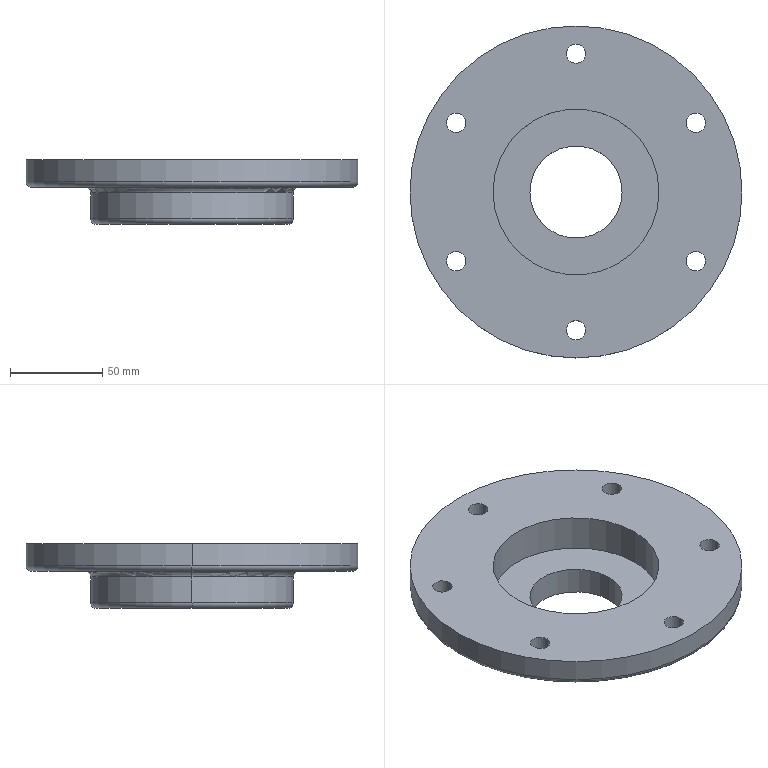Part | SolidWorks | features ICE 2, Extrusion 1, Fillet 1 | 1 solid | 30 faces | box 180 x 180 x 35 mm | volume 406222 mm3 | cylinder 20 | torus 6 | plane 4 | commonest cylinder face diameters 10.5 x12 50 x2 90 x2 110 x2 180 x2
STEP:
#1=CARTESIAN_POINT('',(55.,0.,-17.));
#2=VERTEX_POINT('',#1);
#3=CARTESIAN_POINT('',(-55.,0.,-17.));
#4=VERTEX_POINT('',#3);
#5=CARTESIAN_POINT('',(0.,0.,-17.));
#6=DIRECTION('',(0.,0.,1.));
#7=DIRECTION('',(-1.,0.,0.));
#8=AXIS2_PLACEMENT_3D('',#5,#6,#7);
#9=CIRCLE('',#8,55.);
#10=EDGE_CURVE('',#2,#4,#9,.T.);
#11=ORIENTED_EDGE('',*,*,#10,.F.);
#12=CARTESIAN_POINT('',(52.,0.,-20.));
#13=VERTEX_POINT('',#12);
#14=CARTESIAN_POINT('',(52.,0.,-17.));
#15=DIRECTION('',(0.,1.,0.));
#16=DIRECTION('',(-1.,0.,0.));
#17=AXIS2_PLACEMENT_3D('',#14,#15,#16);
#18=CIRCLE('',#17,3.);
#19=EDGE_CURVE('',#2,#13,#18,.T.);
#20=ORIENTED_EDGE('',*,*,#19,.T.);
#21=CARTESIAN_POINT('',(-52.,0.,-20.));
#22=VERTEX_POINT('',#21);
#23=CARTESIAN_POINT('',(0.,0.,-20.));
#24=DIRECTION('',(0.,0.,-1.));
#25=DIRECTION('',(-1.,0.,0.));
#26=AXIS2_PLACEMENT_3D('',#23,#24,#25);
#27=CIRCLE('',#26,52.);
#28=EDGE_CURVE('',#22,#13,#27,.T.);
#29=ORIENTED_EDGE('',*,*,#28,.F.);
#30=CARTESIAN_POINT('',(-52.,0.,-17.));
#31=DIRECTION('',(0.,-1.,0.));
#32=DIRECTION('',(0.,0.,-1.));
#33=AXIS2_PLACEMENT_3D('',#30,#31,#32);
#34=CIRCLE('',#33,3.);
#35=EDGE_CURVE('',#4,#22,#34,.T.);
#36=ORIENTED_EDGE('',*,*,#35,.F.);
#37=EDGE_LOOP('',(#11,#20,#29,#36));
#38=FACE_OUTER_BOUND('',#37,.T.);
#39=CARTESIAN_POINT('',(0.,0.,-17.));
#40=DIRECTION('',(0.,0.,-1.));
#41=DIRECTION('',(-1.,0.,0.));
#42=AXIS2_PLACEMENT_3D('',#39,#40,#41);
#43=TOROIDAL_SURFACE('',#42,52.,3.);
#44=ADVANCED_FACE('',(#38),#43,.T.);
#45=CARTESIAN_POINT('',(-87.,0.,0.));
#46=VERTEX_POINT('',#45);
#47=CARTESIAN_POINT('',(87.,0.,0.));
#48=VERTEX_POINT('',#47);
#49=CARTESIAN_POINT('',(0.,0.,0.));
#50=DIRECTION('',(0.,0.,-1.));
#51=DIRECTION('',(1.,0.,0.));
#52=AXIS2_PLACEMENT_3D('',#49,#50,#51);
#53=CIRCLE('',#52,87.);
#54=EDGE_CURVE('',#46,#48,#53,.T.);
#55=ORIENTED_EDGE('',*,*,#54,.F.);
#56=CARTESIAN_POINT('',(-90.,0.,3.));
#57=VERTEX_POINT('',#56);
#58=CARTESIAN_POINT('',(-87.,0.,3.));
#59=DIRECTION('',(0.,1.,0.));
#60=DIRECTION('',(-1.,0.,0.));
#61=AXIS2_PLACEMENT_3D('',#58,#59,#60);
#62=CIRCLE('',#61,3.);
#63=EDGE_CURVE('',#46,#57,#62,.T.);
#64=ORIENTED_EDGE('',*,*,#63,.T.);
#65=CARTESIAN_POINT('',(90.,0.,3.));
#66=VERTEX_POINT('',#65);
#67=CARTESIAN_POINT('',(0.,0.,3.));
#68=DIRECTION('',(0.,0.,1.));
#69=DIRECTION('',(1.,0.,0.));
#70=AXIS2_PLACEMENT_3D('',#67,#68,#69);
#71=CIRCLE('',#70,90.);
#72=EDGE_CURVE('',#66,#57,#71,.T.);
#73=ORIENTED_EDGE('',*,*,#72,.F.);
#74=CARTESIAN_POINT('',(87.,0.,3.));
#75=DIRECTION('',(0.,-1.,0.));
#76=DIRECTION('',(0.,0.,-1.));
#77=AXIS2_PLACEMENT_3D('',#74,#75,#76);
#78=CIRCLE('',#77,3.);
#79=EDGE_CURVE('',#48,#66,#78,.T.);
#80=ORIENTED_EDGE('',*,*,#79,.F.);
#81=EDGE_LOOP('',(#55,#64,#73,#80));
#82=FACE_OUTER_BOUND('',#81,.T.);
#83=CARTESIAN_POINT('',(0.,0.,3.));
#84=DIRECTION('',(0.,0.,1.));
#85=DIRECTION('',(1.,0.,0.));
#86=AXIS2_PLACEMENT_3D('',#83,#84,#85);
#87=TOROIDAL_SURFACE('',#86,87.,3.);
#88=ADVANCED_FACE('',(#82),#87,.T.);
#89=CARTESIAN_POINT('',(-58.,0.,0.));
#90=VERTEX_POINT('',#89);
#91=CARTESIAN_POINT('',(58.,0.,0.));
#92=VERTEX_POINT('',#91);
#93=CARTESIAN_POINT('',(0.,0.,0.));
#94=DIRECTION('',(0.,0.,1.));
#95=DIRECTION('',(1.,0.,0.));
#96=AXIS2_PLACEMENT_3D('',#93,#94,#95);
#97=CIRCLE('',#96,58.);
#98=EDGE_CURVE('',#90,#92,#97,.T.);
#99=ORIENTED_EDGE('',*,*,#98,.F.);
#100=CARTESIAN_POINT('',(-55.,0.,-3.));
#101=VERTEX_POINT('',#100);
#102=CARTESIAN_POINT('',(-58.,0.,-3.));
#103=DIRECTION('',(0.,1.,0.));
#104=DIRECTION('',(-1.,0.,0.));
#105=AXIS2_PLACEMENT_3D('',#102,#103,#104);
#106=CIRCLE('',#105,3.);
#107=EDGE_CURVE('',#90,#101,#106,.T.);
#108=ORIENTED_EDGE('',*,*,#107,.T.);
#109=CARTESIAN_POINT('',(55.,0.,-3.));
#110=VERTEX_POINT('',#109);
#111=CARTESIAN_POINT('',(0.,0.,-3.));
#112=DIRECTION('',(0.,0.,-1.));
#113=DIRECTION('',(1.,0.,0.));
#114=AXIS2_PLACEMENT_3D('',#111,#112,#113);
#115=CIRCLE('',#114,55.);
#116=EDGE_CURVE('',#110,#101,#115,.T.);
#117=ORIENTED_EDGE('',*,*,#116,.F.);
#118=CARTESIAN_POINT('',(58.,0.,-3.));
#119=DIRECTION('',(0.,-1.,0.));
#120=DIRECTION('',(0.,0.,-1.));
#121=AXIS2_PLACEMENT_3D('',#118,#119,#120);
#122=CIRCLE('',#121,3.);
#123=EDGE_CURVE('',#92,#110,#122,.T.);
#124=ORIENTED_EDGE('',*,*,#123,.F.);
#125=EDGE_LOOP('',(#99,#108,#117,#124));
#126=FACE_OUTER_BOUND('',#125,.T.);
#127=CARTESIAN_POINT('',(0.,0.,-3.));
#128=DIRECTION('',(0.,0.,1.));
#129=DIRECTION('',(1.,0.,0.));
#130=AXIS2_PLACEMENT_3D('',#127,#128,#129);
#131=TOROIDAL_SURFACE('',#130,58.,3.);
#132=ADVANCED_FACE('',(#126),#131,.F.);
#133=CARTESIAN_POINT('',(-45.,0.,-5.));
#134=VERTEX_POINT('',#133);
#135=CARTESIAN_POINT('',(45.,0.,-5.));
#136=VERTEX_POINT('',#135);
#137=CARTESIAN_POINT('',(0.,0.,-5.));
#138=DIRECTION('',(0.,0.,1.));
#139=DIRECTION('',(1.,0.,0.));
#140=AXIS2_PLACEMENT_3D('',#137,#138,#139);
#141=CIRCLE('',#140,45.);
#142=EDGE_CURVE('',#134,#136,#141,.T.);
#143=ORIENTED_EDGE('',*,*,#142,.F.);
#144=CARTESIAN_POINT('',(-45.,0.,15.));
#145=VERTEX_POINT('',#144);
#146=CARTESIAN_POINT('',(-45.,0.,-5.));
#147=DIRECTION('',(0.,0.,1.));
#148=VECTOR('',#147,1000.);
#149=LINE('',#146,#148);
#150=EDGE_CURVE('',#134,#145,#149,.T.);
#151=ORIENTED_EDGE('',*,*,#150,.T.);
#152=CARTESIAN_POINT('',(45.,0.,15.));
#153=VERTEX_POINT('',#152);
#154=CARTESIAN_POINT('',(0.,0.,15.));
#155=DIRECTION('',(0.,0.,1.));
#156=DIRECTION('',(1.,0.,0.));
#157=AXIS2_PLACEMENT_3D('',#154,#155,#156);
#158=CIRCLE('',#157,45.);
#159=EDGE_CURVE('',#145,#153,#158,.T.);
#160=ORIENTED_EDGE('',*,*,#159,.T.);
#161=CARTESIAN_POINT('',(45.,0.,-5.));
#162=DIRECTION('',(0.,0.,1.));
#163=VECTOR('',#162,1000.);
#164=LINE('',#161,#163);
#165=EDGE_CURVE('',#136,#153,#164,.T.);
#166=ORIENTED_EDGE('',*,*,#165,.F.);
#167=EDGE_LOOP('',(#143,#151,#160,#166));
#168=FACE_OUTER_BOUND('',#167,.T.);
#169=CARTESIAN_POINT('',(0.,0.,-5.));
#170=DIRECTION('',(0.,0.,1.));
#171=DIRECTION('',(1.,0.,0.));
#172=AXIS2_PLACEMENT_3D('',#169,#170,#171);
#173=CYLINDRICAL_SURFACE('',#172,45.);
#174=ADVANCED_FACE('',(#168),#173,.F.);
#175=ORIENTED_EDGE('',*,*,#10,.T.);
#176=CARTESIAN_POINT('',(-55.,0.,-20.));
#177=DIRECTION('',(0.,0.,1.));
#178=VECTOR('',#177,1000.);
#179=LINE('',#176,#178);
#180=EDGE_CURVE('',#4,#101,#179,.T.);
#181=ORIENTED_EDGE('',*,*,#180,.T.);
#182=CARTESIAN_POINT('',(0.,0.,-3.));
#183=DIRECTION('',(0.,0.,-1.));
#184=DIRECTION('',(1.,0.,0.));
#185=AXIS2_PLACEMENT_3D('',#182,#183,#184);
#186=CIRCLE('',#185,55.);
#187=EDGE_CURVE('',#101,#110,#186,.T.);
#188=ORIENTED_EDGE('',*,*,#187,.T.);
#189=CARTESIAN_POINT('',(55.,0.,-20.));
#190=DIRECTION('',(0.,0.,1.));
#191=VECTOR('',#190,1000.);
#192=LINE('',#189,#191);
#193=EDGE_CURVE('',#2,#110,#192,.T.);
#194=ORIENTED_EDGE('',*,*,#193,.F.);
#195=EDGE_LOOP('',(#175,#181,#188,#194));
#196=FACE_OUTER_BOUND('',#195,.T.);
#197=CARTESIAN_POINT('',(0.,0.,-20.));
#198=DIRECTION('',(0.,0.,1.));
#199=DIRECTION('',(1.,0.,0.));
#200=AXIS2_PLACEMENT_3D('',#197,#198,#199);
#201=CYLINDRICAL_SURFACE('',#200,55.);
#202=ADVANCED_FACE('',(#196),#201,.T.);
#203=CARTESIAN_POINT('',(-70.202,37.5,15.));
#204=VERTEX_POINT('',#203);
#205=CARTESIAN_POINT('',(-59.702,37.5,15.));
#206=VERTEX_POINT('',#205);
#207=CARTESIAN_POINT('',(-64.952,37.5,15.));
#208=DIRECTION('',(0.,0.,1.));
#209=DIRECTION('',(1.,0.,0.));
#210=AXIS2_PLACEMENT_3D('',#207,#208,#209);
#211=CIRCLE('',#210,5.25);
#212=EDGE_CURVE('',#204,#206,#211,.T.);
#213=ORIENTED_EDGE('',*,*,#212,.T.);
#214=CARTESIAN_POINT('',(-59.702,37.5,0.));
#215=VERTEX_POINT('',#214);
#216=CARTESIAN_POINT('',(-59.702,37.5,15.));
#217=DIRECTION('',(0.,0.,-1.));
#218=VECTOR('',#217,1000.);
#219=LINE('',#216,#218);
#220=EDGE_CURVE('',#206,#215,#219,.T.);
#221=ORIENTED_EDGE('',*,*,#220,.T.);
#222=CARTESIAN_POINT('',(-70.202,37.5,0.));
#223=VERTEX_POINT('',#222);
#224=CARTESIAN_POINT('',(-64.952,37.5,0.));
#225=DIRECTION('',(0.,0.,1.));
#226=DIRECTION('',(1.,0.,0.));
#227=AXIS2_PLACEMENT_3D('',#224,#225,#226);
#228=CIRCLE('',#227,5.25);
#229=EDGE_CURVE('',#223,#215,#228,.T.);
#230=ORIENTED_EDGE('',*,*,#229,.F.);
#231=CARTESIAN_POINT('',(-70.202,37.5,15.));
#232=DIRECTION('',(0.,0.,-1.));
#233=VECTOR('',#232,1000.);
#234=LINE('',#231,#233);
#235=EDGE_CURVE('',#204,#223,#234,.T.);
#236=ORIENTED_EDGE('',*,*,#235,.F.);
#237=EDGE_LOOP('',(#213,#221,#230,#236));
#238=FACE_OUTER_BOUND('',#237,.T.);
#239=CARTESIAN_POINT('',(-64.952,37.5,15.));
#240=DIRECTION('',(0.,0.,-1.));
#241=DIRECTION('',(-1.,0.,0.));
#242=AXIS2_PLACEMENT_3D('',#239,#240,#241);
#243=CYLINDRICAL_SURFACE('',#242,5.25);
#244=ADVANCED_FACE('',(#238),#243,.F.);
#245=CARTESIAN_POINT('',(-70.202,-37.5,15.));
#246=VERTEX_POINT('',#245);
#247=CARTESIAN_POINT('',(-59.702,-37.5,15.));
#248=VERTEX_POINT('',#247);
#249=CARTESIAN_POINT('',(-64.952,-37.5,15.));
#250=DIRECTION('',(0.,0.,1.));
#251=DIRECTION('',(1.,0.,0.));
#252=AXIS2_PLACEMENT_3D('',#249,#250,#251);
#253=CIRCLE('',#252,5.25);
#254=EDGE_CURVE('',#246,#248,#253,.T.);
#255=ORIENTED_EDGE('',*,*,#254,.T.);
#256=CARTESIAN_POINT('',(-59.702,-37.5,0.));
#257=VERTEX_POINT('',#256);
#258=CARTESIAN_POINT('',(-59.702,-37.5,15.));
#259=DIRECTION('',(0.,0.,-1.));
#260=VECTOR('',#259,1000.);
#261=LINE('',#258,#260);
#262=EDGE_CURVE('',#248,#257,#261,.T.);
#263=ORIENTED_EDGE('',*,*,#262,.T.);
#264=CARTESIAN_POINT('',(-70.202,-37.5,0.));
#265=VERTEX_POINT('',#264);
#266=CARTESIAN_POINT('',(-64.952,-37.5,0.));
#267=DIRECTION('',(0.,0.,1.));
#268=DIRECTION('',(1.,0.,0.));
#269=AXIS2_PLACEMENT_3D('',#266,#267,#268);
#270=CIRCLE('',#269,5.25);
#271=EDGE_CURVE('',#265,#257,#270,.T.);
#272=ORIENTED_EDGE('',*,*,#271,.F.);
#273=CARTESIAN_POINT('',(-70.202,-37.5,15.));
#274=DIRECTION('',(0.,0.,-1.));
#275=VECTOR('',#274,1000.);
#276=LINE('',#273,#275);
#277=EDGE_CURVE('',#246,#265,#276,.T.);
#278=ORIENTED_EDGE('',*,*,#277,.F.);
#279=EDGE_LOOP('',(#255,#263,#272,#278));
#280=FACE_OUTER_BOUND('',#279,.T.);
#281=CARTESIAN_POINT('',(-64.952,-37.5,15.));
#282=DIRECTION('',(0.,0.,-1.));
#283=DIRECTION('',(-1.,0.,0.));
#284=AXIS2_PLACEMENT_3D('',#281,#282,#283);
#285=CYLINDRICAL_SURFACE('',#284,5.25);
#286=ADVANCED_FACE('',(#280),#285,.F.);
#287=CARTESIAN_POINT('',(-5.25,-75.,15.));
#288=VERTEX_POINT('',#287);
#289=CARTESIAN_POINT('',(5.25,-75.,15.));
#290=VERTEX_POINT('',#289);
#291=CARTESIAN_POINT('',(0.,-75.,15.));
#292=DIRECTION('',(0.,0.,1.));
#293=DIRECTION('',(1.,0.,0.));
#294=AXIS2_PLACEMENT_3D('',#291,#292,#293);
#295=CIRCLE('',#294,5.25);
#296=EDGE_CURVE('',#288,#290,#295,.T.);
#297=ORIENTED_EDGE('',*,*,#296,.T.);
#298=CARTESIAN_POINT('',(5.25,-75.,0.));
#299=VERTEX_POINT('',#298);
#300=CARTESIAN_POINT('',(5.25,-75.,15.));
#301=DIRECTION('',(0.,0.,-1.));
#302=VECTOR('',#301,1000.);
#303=LINE('',#300,#302);
#304=EDGE_CURVE('',#290,#299,#303,.T.);
#305=ORIENTED_EDGE('',*,*,#304,.T.);
#306=CARTESIAN_POINT('',(-5.25,-75.,0.));
#307=VERTEX_POINT('',#306);
#308=CARTESIAN_POINT('',(0.,-75.,0.));
#309=DIRECTION('',(0.,0.,1.));
#310=DIRECTION('',(1.,0.,0.));
#311=AXIS2_PLACEMENT_3D('',#308,#309,#310);
#312=CIRCLE('',#311,5.25);
#313=EDGE_CURVE('',#307,#299,#312,.T.);
#314=ORIENTED_EDGE('',*,*,#313,.F.);
#315=CARTESIAN_POINT('',(-5.25,-75.,15.));
#316=DIRECTION('',(0.,0.,-1.));
#317=VECTOR('',#316,1000.);
#318=LINE('',#315,#317);
#319=EDGE_CURVE('',#288,#307,#318,.T.);
#320=ORIENTED_EDGE('',*,*,#319,.F.);
#321=EDGE_LOOP('',(#297,#305,#314,#320));
#322=FACE_OUTER_BOUND('',#321,.T.);
#323=CARTESIAN_POINT('',(0.,-75.,15.));
#324=DIRECTION('',(0.,0.,-1.));
#325=DIRECTION('',(-1.,0.,0.));
#326=AXIS2_PLACEMENT_3D('',#323,#324,#325);
#327=CYLINDRICAL_SURFACE('',#326,5.25);
#328=ADVANCED_FACE('',(#322),#327,.F.);
#329=CARTESIAN_POINT('',(59.702,-37.5,15.));
#330=VERTEX_POINT('',#329);
#331=CARTESIAN_POINT('',(70.202,-37.5,15.));
#332=VERTEX_POINT('',#331);
#333=CARTESIAN_POINT('',(64.952,-37.5,15.));
#334=DIRECTION('',(0.,0.,1.));
#335=DIRECTION('',(1.,0.,0.));
#336=AXIS2_PLACEMENT_3D('',#333,#334,#335);
#337=CIRCLE('',#336,5.25);
#338=EDGE_CURVE('',#330,#332,#337,.T.);
#339=ORIENTED_EDGE('',*,*,#338,.T.);
#340=CARTESIAN_POINT('',(70.202,-37.5,0.));
#341=VERTEX_POINT('',#340);
#342=CARTESIAN_POINT('',(70.202,-37.5,15.));
#343=DIRECTION('',(0.,0.,-1.));
#344=VECTOR('',#343,1000.);
#345=LINE('',#342,#344);
#346=EDGE_CURVE('',#332,#341,#345,.T.);
#347=ORIENTED_EDGE('',*,*,#346,.T.);
#348=CARTESIAN_POINT('',(59.702,-37.5,0.));
#349=VERTEX_POINT('',#348);
#350=CARTESIAN_POINT('',(64.952,-37.5,0.));
#351=DIRECTION('',(0.,0.,1.));
#352=DIRECTION('',(1.,0.,0.));
#353=AXIS2_PLACEMENT_3D('',#350,#351,#352);
#354=CIRCLE('',#353,5.25);
#355=EDGE_CURVE('',#349,#341,#354,.T.);
#356=ORIENTED_EDGE('',*,*,#355,.F.);
#357=CARTESIAN_POINT('',(59.702,-37.5,15.));
#358=DIRECTION('',(0.,0.,-1.));
#359=VECTOR('',#358,1000.);
#360=LINE('',#357,#359);
#361=EDGE_CURVE('',#330,#349,#360,.T.);
#362=ORIENTED_EDGE('',*,*,#361,.F.);
#363=EDGE_LOOP('',(#339,#347,#356,#362));
#364=FACE_OUTER_BOUND('',#363,.T.);
#365=CARTESIAN_POINT('',(64.952,-37.5,15.));
#366=DIRECTION('',(0.,0.,-1.));
#367=DIRECTION('',(-1.,0.,0.));
#368=AXIS2_PLACEMENT_3D('',#365,#366,#367);
#369=CYLINDRICAL_SURFACE('',#368,5.25);
#370=ADVANCED_FACE('',(#364),#369,.F.);
#371=CARTESIAN_POINT('',(59.702,37.5,15.));
#372=VERTEX_POINT('',#371);
#373=CARTESIAN_POINT('',(70.202,37.5,15.));
#374=VERTEX_POINT('',#373);
#375=CARTESIAN_POINT('',(64.952,37.5,15.));
#376=DIRECTION('',(0.,0.,1.));
#377=DIRECTION('',(1.,0.,0.));
#378=AXIS2_PLACEMENT_3D('',#375,#376,#377);
#379=CIRCLE('',#378,5.25);
#380=EDGE_CURVE('',#372,#374,#379,.T.);
#381=ORIENTED_EDGE('',*,*,#380,.T.);
#382=CARTESIAN_POINT('',(70.202,37.5,0.));
#383=VERTEX_POINT('',#382);
#384=CARTESIAN_POINT('',(70.202,37.5,15.));
#385=DIRECTION('',(0.,0.,-1.));
#386=VECTOR('',#385,1000.);
#387=LINE('',#384,#386);
#388=EDGE_CURVE('',#374,#383,#387,.T.);
#389=ORIENTED_EDGE('',*,*,#388,.T.);
#390=CARTESIAN_POINT('',(59.702,37.5,0.));
#391=VERTEX_POINT('',#390);
#392=CARTESIAN_POINT('',(64.952,37.5,0.));
#393=DIRECTION('',(0.,0.,1.));
#394=DIRECTION('',(1.,0.,0.));
#395=AXIS2_PLACEMENT_3D('',#392,#393,#394);
#396=CIRCLE('',#395,5.25);
#397=EDGE_CURVE('',#391,#383,#396,.T.);
#398=ORIENTED_EDGE('',*,*,#397,.F.);
#399=CARTESIAN_POINT('',(59.702,37.5,15.));
#400=DIRECTION('',(0.,0.,-1.));
#401=VECTOR('',#400,1000.);
#402=LINE('',#399,#401);
#403=EDGE_CURVE('',#372,#391,#402,.T.);
#404=ORIENTED_EDGE('',*,*,#403,.F.);
#405=EDGE_LOOP('',(#381,#389,#398,#404));
#406=FACE_OUTER_BOUND('',#405,.T.);
#407=CARTESIAN_POINT('',(64.952,37.5,15.));
#408=DIRECTION('',(0.,0.,-1.));
#409=DIRECTION('',(-1.,0.,0.));
#410=AXIS2_PLACEMENT_3D('',#407,#408,#409);
#411=CYLINDRICAL_SURFACE('',#410,5.25);
#412=ADVANCED_FACE('',(#406),#411,.F.);
#413=CARTESIAN_POINT('',(-5.25,75.,15.));
#414=VERTEX_POINT('',#413);
#415=CARTESIAN_POINT('',(5.25,75.,15.));
#416=VERTEX_POINT('',#415);
#417=CARTESIAN_POINT('',(0.,75.,15.));
#418=DIRECTION('',(0.,0.,1.));
#419=DIRECTION('',(1.,0.,0.));
#420=AXIS2_PLACEMENT_3D('',#417,#418,#419);
#421=CIRCLE('',#420,5.25);
#422=EDGE_CURVE('',#414,#416,#421,.T.);
#423=ORIENTED_EDGE('',*,*,#422,.T.);
#424=CARTESIAN_POINT('',(5.25,75.,0.));
#425=VERTEX_POINT('',#424);
#426=CARTESIAN_POINT('',(5.25,75.,15.));
#427=DIRECTION('',(0.,0.,-1.));
#428=VECTOR('',#427,1000.);
#429=LINE('',#426,#428);
#430=EDGE_CURVE('',#416,#425,#429,.T.);
#431=ORIENTED_EDGE('',*,*,#430,.T.);
#432=CARTESIAN_POINT('',(-5.25,75.,0.));
#433=VERTEX_POINT('',#432);
#434=CARTESIAN_POINT('',(0.,75.,0.));
#435=DIRECTION('',(0.,0.,1.));
#436=DIRECTION('',(1.,0.,0.));
#437=AXIS2_PLACEMENT_3D('',#434,#435,#436);
#438=CIRCLE('',#437,5.25);
#439=EDGE_CURVE('',#433,#425,#438,.T.);
#440=ORIENTED_EDGE('',*,*,#439,.F.);
#441=CARTESIAN_POINT('',(-5.25,75.,15.));
#442=DIRECTION('',(0.,0.,-1.));
#443=VECTOR('',#442,1000.);
#444=LINE('',#441,#443);
#445=EDGE_CURVE('',#414,#433,#444,.T.);
#446=ORIENTED_EDGE('',*,*,#445,.F.);
#447=EDGE_LOOP('',(#423,#431,#440,#446));
#448=FACE_OUTER_BOUND('',#447,.T.);
#449=CARTESIAN_POINT('',(0.,75.,15.));
#450=DIRECTION('',(0.,0.,-1.));
#451=DIRECTION('',(-1.,0.,0.));
#452=AXIS2_PLACEMENT_3D('',#449,#450,#451);
#453=CYLINDRICAL_SURFACE('',#452,5.25);
#454=ADVANCED_FACE('',(#448),#453,.F.);
#455=CARTESIAN_POINT('',(90.,0.,15.));
#456=VERTEX_POINT('',#455);
#457=CARTESIAN_POINT('',(-90.,0.,15.));
#458=VERTEX_POINT('',#457);
#459=CARTESIAN_POINT('',(0.,0.,15.));
#460=DIRECTION('',(0.,0.,1.));
#461=DIRECTION('',(1.,0.,0.));
#462=AXIS2_PLACEMENT_3D('',#459,#460,#461);
#463=CIRCLE('',#462,90.);
#464=EDGE_CURVE('',#456,#458,#463,.T.);
#465=ORIENTED_EDGE('',*,*,#464,.F.);
#466=CARTESIAN_POINT('',(90.,0.,15.));
#467=DIRECTION('',(0.,0.,-1.));
#468=VECTOR('',#467,1000.);
#469=LINE('',#466,#468);
#470=EDGE_CURVE('',#456,#66,#469,.T.);
#471=ORIENTED_EDGE('',*,*,#470,.T.);
#472=ORIENTED_EDGE('',*,*,#72,.T.);
#473=CARTESIAN_POINT('',(-90.,0.,15.));
#474=DIRECTION('',(0.,0.,-1.));
#475=VECTOR('',#474,1000.);
#476=LINE('',#473,#475);
#477=EDGE_CURVE('',#458,#57,#476,.T.);
#478=ORIENTED_EDGE('',*,*,#477,.F.);
#479=EDGE_LOOP('',(#465,#471,#472,#478));
#480=FACE_OUTER_BOUND('',#479,.T.);
#481=CARTESIAN_POINT('',(0.,0.,15.));
#482=DIRECTION('',(0.,0.,-1.));
#483=DIRECTION('',(-1.,0.,0.));
#484=AXIS2_PLACEMENT_3D('',#481,#482,#483);
#485=CYLINDRICAL_SURFACE('',#484,90.);
#486=ADVANCED_FACE('',(#480),#485,.T.);
#487=CARTESIAN_POINT('',(-25.,0.,-5.));
#488=VERTEX_POINT('',#487);
#489=CARTESIAN_POINT('',(25.,0.,-5.));
#490=VERTEX_POINT('',#489);
#491=CARTESIAN_POINT('',(0.,0.,-5.));
#492=DIRECTION('',(0.,0.,1.));
#493=DIRECTION('',(1.,0.,0.));
#494=AXIS2_PLACEMENT_3D('',#491,#492,#493);
#495=CIRCLE('',#494,25.);
#496=EDGE_CURVE('',#488,#490,#495,.T.);
#497=ORIENTED_EDGE('',*,*,#496,.T.);
#498=CARTESIAN_POINT('',(25.,0.,-20.));
#499=VERTEX_POINT('',#498);
#500=CARTESIAN_POINT('',(25.,0.,15.));
#501=DIRECTION('',(0.,0.,-1.));
#502=VECTOR('',#501,1000.);
#503=LINE('',#500,#502);
#504=EDGE_CURVE('',#490,#499,#503,.T.);
#505=ORIENTED_EDGE('',*,*,#504,.T.);
#506=CARTESIAN_POINT('',(-25.,0.,-20.));
#507=VERTEX_POINT('',#506);
#508=CARTESIAN_POINT('',(0.,0.,-20.));
#509=DIRECTION('',(0.,0.,-1.));
#510=DIRECTION('',(-1.,0.,0.));
#511=AXIS2_PLACEMENT_3D('',#508,#509,#510);
#512=CIRCLE('',#511,25.);
#513=EDGE_CURVE('',#499,#507,#512,.T.);
#514=ORIENTED_EDGE('',*,*,#513,.T.);
#515=CARTESIAN_POINT('',(-25.,0.,15.));
#516=DIRECTION('',(0.,0.,-1.));
#517=VECTOR('',#516,1000.);
#518=LINE('',#515,#517);
#519=EDGE_CURVE('',#488,#507,#518,.T.);
#520=ORIENTED_EDGE('',*,*,#519,.F.);
#521=EDGE_LOOP('',(#497,#505,#514,#520));
#522=FACE_OUTER_BOUND('',#521,.T.);
#523=CARTESIAN_POINT('',(0.,0.,15.));
#524=DIRECTION('',(0.,0.,-1.));
#525=DIRECTION('',(-1.,0.,0.));
#526=AXIS2_PLACEMENT_3D('',#523,#524,#525);
#527=CYLINDRICAL_SURFACE('',#526,25.);
#528=ADVANCED_FACE('',(#522),#527,.F.);
#529=ORIENTED_EDGE('',*,*,#504,.F.);
#530=CARTESIAN_POINT('',(0.,0.,-5.));
#531=DIRECTION('',(0.,0.,1.));
#532=DIRECTION('',(1.,0.,0.));
#533=AXIS2_PLACEMENT_3D('',#530,#531,#532);
#534=CIRCLE('',#533,25.);
#535=EDGE_CURVE('',#490,#488,#534,.T.);
#536=ORIENTED_EDGE('',*,*,#535,.T.);
#537=ORIENTED_EDGE('',*,*,#519,.T.);
#538=CARTESIAN_POINT('',(0.,0.,-20.));
#539=DIRECTION('',(0.,0.,-1.));
#540=DIRECTION('',(-1.,0.,0.));
#541=AXIS2_PLACEMENT_3D('',#538,#539,#540);
#542=CIRCLE('',#541,25.);
#543=EDGE_CURVE('',#507,#499,#542,.T.);
#544=ORIENTED_EDGE('',*,*,#543,.T.);
#545=EDGE_LOOP('',(#529,#536,#537,#544));
#546=FACE_OUTER_BOUND('',#545,.T.);
#547=CARTESIAN_POINT('',(0.,0.,15.));
#548=DIRECTION('',(0.,0.,-1.));
#549=DIRECTION('',(-1.,0.,0.));
#550=AXIS2_PLACEMENT_3D('',#547,#548,#549);
#551=CYLINDRICAL_SURFACE('',#550,25.);
#552=ADVANCED_FACE('',(#546),#551,.F.);
#553=CARTESIAN_POINT('',(0.,0.,0.));
#554=DIRECTION('',(0.,0.,1.));
#555=DIRECTION('',(1.,0.,0.));
#556=AXIS2_PLACEMENT_3D('',#553,#554,#555);
#557=CIRCLE('',#556,58.);
#558=EDGE_CURVE('',#92,#90,#557,.T.);
#559=ORIENTED_EDGE('',*,*,#558,.T.);
#560=ORIENTED_EDGE('',*,*,#98,.T.);
#561=EDGE_LOOP('',(#559,#560));
#562=FACE_BOUND('',#561,.T.);
#563=CARTESIAN_POINT('',(0.,0.,0.));
#564=DIRECTION('',(0.,0.,-1.));
#565=DIRECTION('',(1.,0.,0.));
#566=AXIS2_PLACEMENT_3D('',#563,#564,#565);
#567=CIRCLE('',#566,87.);
#568=EDGE_CURVE('',#48,#46,#567,.T.);
#569=ORIENTED_EDGE('',*,*,#568,.T.);
#570=ORIENTED_EDGE('',*,*,#54,.T.);
#571=EDGE_LOOP('',(#569,#570));
#572=FACE_OUTER_BOUND('',#571,.T.);
#573=ORIENTED_EDGE('',*,*,#229,.T.);
#574=CARTESIAN_POINT('',(-64.952,37.5,0.));
#575=DIRECTION('',(0.,0.,1.));
#576=DIRECTION('',(1.,0.,0.));
#577=AXIS2_PLACEMENT_3D('',#574,#575,#576);
#578=CIRCLE('',#577,5.25);
#579=EDGE_CURVE('',#215,#223,#578,.T.);
#580=ORIENTED_EDGE('',*,*,#579,.T.);
#581=EDGE_LOOP('',(#573,#580));
#582=FACE_BOUND('',#581,.T.);
#583=ORIENTED_EDGE('',*,*,#271,.T.);
#584=CARTESIAN_POINT('',(-64.952,-37.5,0.));
#585=DIRECTION('',(0.,0.,1.));
#586=DIRECTION('',(1.,0.,0.));
#587=AXIS2_PLACEMENT_3D('',#584,#585,#586);
#588=CIRCLE('',#587,5.25);
#589=EDGE_CURVE('',#257,#265,#588,.T.);
#590=ORIENTED_EDGE('',*,*,#589,.T.);
#591=EDGE_LOOP('',(#583,#590));
#592=FACE_BOUND('',#591,.T.);
#593=ORIENTED_EDGE('',*,*,#313,.T.);
#594=CARTESIAN_POINT('',(0.,-75.,0.));
#595=DIRECTION('',(0.,0.,1.));
#596=DIRECTION('',(1.,0.,0.));
#597=AXIS2_PLACEMENT_3D('',#594,#595,#596);
#598=CIRCLE('',#597,5.25);
#599=EDGE_CURVE('',#299,#307,#598,.T.);
#600=ORIENTED_EDGE('',*,*,#599,.T.);
#601=EDGE_LOOP('',(#593,#600));
#602=FACE_BOUND('',#601,.T.);
#603=ORIENTED_EDGE('',*,*,#355,.T.);
#604=CARTESIAN_POINT('',(64.952,-37.5,0.));
#605=DIRECTION('',(0.,0.,1.));
#606=DIRECTION('',(1.,0.,0.));
#607=AXIS2_PLACEMENT_3D('',#604,#605,#606);
#608=CIRCLE('',#607,5.25);
#609=EDGE_CURVE('',#341,#349,#608,.T.);
#610=ORIENTED_EDGE('',*,*,#609,.T.);
#611=EDGE_LOOP('',(#603,#610));
#612=FACE_BOUND('',#611,.T.);
#613=ORIENTED_EDGE('',*,*,#397,.T.);
#614=CARTESIAN_POINT('',(64.952,37.5,0.));
#615=DIRECTION('',(0.,0.,1.));
#616=DIRECTION('',(1.,0.,0.));
#617=AXIS2_PLACEMENT_3D('',#614,#615,#616);
#618=CIRCLE('',#617,5.25);
#619=EDGE_CURVE('',#383,#391,#618,.T.);
#620=ORIENTED_EDGE('',*,*,#619,.T.);
#621=EDGE_LOOP('',(#613,#620));
#622=FACE_BOUND('',#621,.T.);
#623=ORIENTED_EDGE('',*,*,#439,.T.);
#624=CARTESIAN_POINT('',(0.,75.,0.));
#625=DIRECTION('',(0.,0.,1.));
#626=DIRECTION('',(1.,0.,0.));
#627=AXIS2_PLACEMENT_3D('',#624,#625,#626);
#628=CIRCLE('',#627,5.25);
#629=EDGE_CURVE('',#425,#433,#628,.T.);
#630=ORIENTED_EDGE('',*,*,#629,.T.);
#631=EDGE_LOOP('',(#623,#630));
#632=FACE_BOUND('',#631,.T.);
#633=CARTESIAN_POINT('',(0.,0.,0.));
#634=DIRECTION('',(0.,0.,1.));
#635=DIRECTION('',(1.,0.,0.));
#636=AXIS2_PLACEMENT_3D('',#633,#634,#635);
#637=PLANE('',#636);
#638=ADVANCED_FACE('',(#562,#572,#582,#592,#602,#612,#622,#632),#637,.F.);
#639=CARTESIAN_POINT('',(0.,0.,15.));
#640=DIRECTION('',(0.,0.,1.));
#641=DIRECTION('',(1.,0.,0.));
#642=AXIS2_PLACEMENT_3D('',#639,#640,#641);
#643=CIRCLE('',#642,45.);
#644=EDGE_CURVE('',#153,#145,#643,.T.);
#645=ORIENTED_EDGE('',*,*,#644,.F.);
#646=ORIENTED_EDGE('',*,*,#159,.F.);
#647=EDGE_LOOP('',(#645,#646));
#648=FACE_BOUND('',#647,.T.);
#649=ORIENTED_EDGE('',*,*,#254,.F.);
#650=CARTESIAN_POINT('',(-64.952,-37.5,15.));
#651=DIRECTION('',(0.,0.,1.));
#652=DIRECTION('',(1.,0.,0.));
#653=AXIS2_PLACEMENT_3D('',#650,#651,#652);
#654=CIRCLE('',#653,5.25);
#655=EDGE_CURVE('',#248,#246,#654,.T.);
#656=ORIENTED_EDGE('',*,*,#655,.F.);
#657=EDGE_LOOP('',(#649,#656));
#658=FACE_BOUND('',#657,.T.);
#659=ORIENTED_EDGE('',*,*,#338,.F.);
#660=CARTESIAN_POINT('',(64.952,-37.5,15.));
#661=DIRECTION('',(0.,0.,1.));
#662=DIRECTION('',(1.,0.,0.));
#663=AXIS2_PLACEMENT_3D('',#660,#661,#662);
#664=CIRCLE('',#663,5.25);
#665=EDGE_CURVE('',#332,#330,#664,.T.);
#666=ORIENTED_EDGE('',*,*,#665,.F.);
#667=EDGE_LOOP('',(#659,#666));
#668=FACE_BOUND('',#667,.T.);
#669=ORIENTED_EDGE('',*,*,#422,.F.);
#670=CARTESIAN_POINT('',(0.,75.,15.));
#671=DIRECTION('',(0.,0.,1.));
#672=DIRECTION('',(1.,0.,0.));
#673=AXIS2_PLACEMENT_3D('',#670,#671,#672);
#674=CIRCLE('',#673,5.25);
#675=EDGE_CURVE('',#416,#414,#674,.T.);
#676=ORIENTED_EDGE('',*,*,#675,.F.);
#677=EDGE_LOOP('',(#669,#676));
#678=FACE_BOUND('',#677,.T.);
#679=CARTESIAN_POINT('',(0.,0.,15.));
#680=DIRECTION('',(0.,0.,1.));
#681=DIRECTION('',(1.,0.,0.));
#682=AXIS2_PLACEMENT_3D('',#679,#680,#681);
#683=CIRCLE('',#682,90.);
#684=EDGE_CURVE('',#458,#456,#683,.T.);
#685=ORIENTED_EDGE('',*,*,#684,.T.);
#686=ORIENTED_EDGE('',*,*,#464,.T.);
#687=EDGE_LOOP('',(#685,#686));
#688=FACE_OUTER_BOUND('',#687,.T.);
#689=ORIENTED_EDGE('',*,*,#380,.F.);
#690=CARTESIAN_POINT('',(64.952,37.5,15.));
#691=DIRECTION('',(0.,0.,1.));
#692=DIRECTION('',(1.,0.,0.));
#693=AXIS2_PLACEMENT_3D('',#690,#691,#692);
#694=CIRCLE('',#693,5.25);
#695=EDGE_CURVE('',#374,#372,#694,.T.);
#696=ORIENTED_EDGE('',*,*,#695,.F.);
#697=EDGE_LOOP('',(#689,#696));
#698=FACE_BOUND('',#697,.T.);
#699=ORIENTED_EDGE('',*,*,#296,.F.);
#700=CARTESIAN_POINT('',(0.,-75.,15.));
#701=DIRECTION('',(0.,0.,1.));
#702=DIRECTION('',(1.,0.,0.));
#703=AXIS2_PLACEMENT_3D('',#700,#701,#702);
#704=CIRCLE('',#703,5.25);
#705=EDGE_CURVE('',#290,#288,#704,.T.);
#706=ORIENTED_EDGE('',*,*,#705,.F.);
#707=EDGE_LOOP('',(#699,#706));
#708=FACE_BOUND('',#707,.T.);
#709=ORIENTED_EDGE('',*,*,#212,.F.);
#710=CARTESIAN_POINT('',(-64.952,37.5,15.));
#711=DIRECTION('',(0.,0.,1.));
#712=DIRECTION('',(1.,0.,0.));
#713=AXIS2_PLACEMENT_3D('',#710,#711,#712);
#714=CIRCLE('',#713,5.25);
#715=EDGE_CURVE('',#206,#204,#714,.T.);
#716=ORIENTED_EDGE('',*,*,#715,.F.);
#717=EDGE_LOOP('',(#709,#716));
#718=FACE_BOUND('',#717,.T.);
#719=CARTESIAN_POINT('',(0.,0.,15.));
#720=DIRECTION('',(0.,0.,1.));
#721=DIRECTION('',(1.,0.,0.));
#722=AXIS2_PLACEMENT_3D('',#719,#720,#721);
#723=PLANE('',#722);
#724=ADVANCED_FACE('',(#648,#658,#668,#678,#688,#698,#708,#718),#723,.T.);
#725=ORIENTED_EDGE('',*,*,#470,.F.);
#726=ORIENTED_EDGE('',*,*,#684,.F.);
#727=ORIENTED_EDGE('',*,*,#477,.T.);
#728=CARTESIAN_POINT('',(0.,0.,3.));
#729=DIRECTION('',(0.,0.,1.));
#730=DIRECTION('',(1.,0.,0.));
#731=AXIS2_PLACEMENT_3D('',#728,#729,#730);
#732=CIRCLE('',#731,90.);
#733=EDGE_CURVE('',#57,#66,#732,.T.);
#734=ORIENTED_EDGE('',*,*,#733,.T.);
#735=EDGE_LOOP('',(#725,#726,#727,#734));
#736=FACE_OUTER_BOUND('',#735,.T.);
#737=CARTESIAN_POINT('',(0.,0.,15.));
#738=DIRECTION('',(0.,0.,-1.));
#739=DIRECTION('',(-1.,0.,0.));
#740=AXIS2_PLACEMENT_3D('',#737,#738,#739);
#741=CYLINDRICAL_SURFACE('',#740,90.);
#742=ADVANCED_FACE('',(#736),#741,.T.);
#743=ORIENTED_EDGE('',*,*,#430,.F.);
#744=ORIENTED_EDGE('',*,*,#675,.T.);
#745=ORIENTED_EDGE('',*,*,#445,.T.);
#746=ORIENTED_EDGE('',*,*,#629,.F.);
#747=EDGE_LOOP('',(#743,#744,#745,#746));
#748=FACE_OUTER_BOUND('',#747,.T.);
#749=CARTESIAN_POINT('',(0.,75.,15.));
#750=DIRECTION('',(0.,0.,-1.));
#751=DIRECTION('',(-1.,0.,0.));
#752=AXIS2_PLACEMENT_3D('',#749,#750,#751);
#753=CYLINDRICAL_SURFACE('',#752,5.25);
#754=ADVANCED_FACE('',(#748),#753,.F.);
#755=ORIENTED_EDGE('',*,*,#388,.F.);
#756=ORIENTED_EDGE('',*,*,#695,.T.);
#757=ORIENTED_EDGE('',*,*,#403,.T.);
#758=ORIENTED_EDGE('',*,*,#619,.F.);
#759=EDGE_LOOP('',(#755,#756,#757,#758));
#760=FACE_OUTER_BOUND('',#759,.T.);
#761=CARTESIAN_POINT('',(64.952,37.5,15.));
#762=DIRECTION('',(0.,0.,-1.));
#763=DIRECTION('',(-1.,0.,0.));
#764=AXIS2_PLACEMENT_3D('',#761,#762,#763);
#765=CYLINDRICAL_SURFACE('',#764,5.25);
#766=ADVANCED_FACE('',(#760),#765,.F.);
#767=ORIENTED_EDGE('',*,*,#346,.F.);
#768=ORIENTED_EDGE('',*,*,#665,.T.);
#769=ORIENTED_EDGE('',*,*,#361,.T.);
#770=ORIENTED_EDGE('',*,*,#609,.F.);
#771=EDGE_LOOP('',(#767,#768,#769,#770));
#772=FACE_OUTER_BOUND('',#771,.T.);
#773=CARTESIAN_POINT('',(64.952,-37.5,15.));
#774=DIRECTION('',(0.,0.,-1.));
#775=DIRECTION('',(-1.,0.,0.));
#776=AXIS2_PLACEMENT_3D('',#773,#774,#775);
#777=CYLINDRICAL_SURFACE('',#776,5.25);
#778=ADVANCED_FACE('',(#772),#777,.F.);
#779=ORIENTED_EDGE('',*,*,#304,.F.);
#780=ORIENTED_EDGE('',*,*,#705,.T.);
#781=ORIENTED_EDGE('',*,*,#319,.T.);
#782=ORIENTED_EDGE('',*,*,#599,.F.);
#783=EDGE_LOOP('',(#779,#780,#781,#782));
#784=FACE_OUTER_BOUND('',#783,.T.);
#785=CARTESIAN_POINT('',(0.,-75.,15.));
#786=DIRECTION('',(0.,0.,-1.));
#787=DIRECTION('',(-1.,0.,0.));
#788=AXIS2_PLACEMENT_3D('',#785,#786,#787);
#789=CYLINDRICAL_SURFACE('',#788,5.25);
#790=ADVANCED_FACE('',(#784),#789,.F.);
#791=ORIENTED_EDGE('',*,*,#262,.F.);
#792=ORIENTED_EDGE('',*,*,#655,.T.);
#793=ORIENTED_EDGE('',*,*,#277,.T.);
#794=ORIENTED_EDGE('',*,*,#589,.F.);
#795=EDGE_LOOP('',(#791,#792,#793,#794));
#796=FACE_OUTER_BOUND('',#795,.T.);
#797=CARTESIAN_POINT('',(-64.952,-37.5,15.));
#798=DIRECTION('',(0.,0.,-1.));
#799=DIRECTION('',(-1.,0.,0.));
#800=AXIS2_PLACEMENT_3D('',#797,#798,#799);
#801=CYLINDRICAL_SURFACE('',#800,5.25);
#802=ADVANCED_FACE('',(#796),#801,.F.);
#803=ORIENTED_EDGE('',*,*,#220,.F.);
#804=ORIENTED_EDGE('',*,*,#715,.T.);
#805=ORIENTED_EDGE('',*,*,#235,.T.);
#806=ORIENTED_EDGE('',*,*,#579,.F.);
#807=EDGE_LOOP('',(#803,#804,#805,#806));
#808=FACE_OUTER_BOUND('',#807,.T.);
#809=CARTESIAN_POINT('',(-64.952,37.5,15.));
#810=DIRECTION('',(0.,0.,-1.));
#811=DIRECTION('',(-1.,0.,0.));
#812=AXIS2_PLACEMENT_3D('',#809,#810,#811);
#813=CYLINDRICAL_SURFACE('',#812,5.25);
#814=ADVANCED_FACE('',(#808),#813,.F.);
#815=ORIENTED_EDGE('',*,*,#28,.T.);
#816=CARTESIAN_POINT('',(0.,0.,-20.));
#817=DIRECTION('',(0.,0.,-1.));
#818=DIRECTION('',(-1.,0.,0.));
#819=AXIS2_PLACEMENT_3D('',#816,#817,#818);
#820=CIRCLE('',#819,52.);
#821=EDGE_CURVE('',#13,#22,#820,.T.);
#822=ORIENTED_EDGE('',*,*,#821,.T.);
#823=EDGE_LOOP('',(#815,#822));
#824=FACE_OUTER_BOUND('',#823,.T.);
#825=ORIENTED_EDGE('',*,*,#543,.F.);
#826=ORIENTED_EDGE('',*,*,#513,.F.);
#827=EDGE_LOOP('',(#825,#826));
#828=FACE_BOUND('',#827,.T.);
#829=CARTESIAN_POINT('',(0.,0.,-20.));
#830=DIRECTION('',(0.,0.,-1.));
#831=DIRECTION('',(-1.,0.,0.));
#832=AXIS2_PLACEMENT_3D('',#829,#830,#831);
#833=PLANE('',#832);
#834=ADVANCED_FACE('',(#824,#828),#833,.T.);
#835=ORIENTED_EDGE('',*,*,#180,.F.);
#836=CARTESIAN_POINT('',(0.,0.,-17.));
#837=DIRECTION('',(0.,0.,1.));
#838=DIRECTION('',(-1.,0.,0.));
#839=AXIS2_PLACEMENT_3D('',#836,#837,#838);
#840=CIRCLE('',#839,55.);
#841=EDGE_CURVE('',#4,#2,#840,.T.);
#842=ORIENTED_EDGE('',*,*,#841,.T.);
#843=ORIENTED_EDGE('',*,*,#193,.T.);
#844=ORIENTED_EDGE('',*,*,#116,.T.);
#845=EDGE_LOOP('',(#835,#842,#843,#844));
#846=FACE_OUTER_BOUND('',#845,.T.);
#847=CARTESIAN_POINT('',(0.,0.,-20.));
#848=DIRECTION('',(0.,0.,1.));
#849=DIRECTION('',(1.,0.,0.));
#850=AXIS2_PLACEMENT_3D('',#847,#848,#849);
#851=CYLINDRICAL_SURFACE('',#850,55.);
#852=ADVANCED_FACE('',(#846),#851,.T.);
#853=ORIENTED_EDGE('',*,*,#150,.F.);
#854=CARTESIAN_POINT('',(0.,0.,-5.));
#855=DIRECTION('',(0.,0.,1.));
#856=DIRECTION('',(1.,0.,0.));
#857=AXIS2_PLACEMENT_3D('',#854,#855,#856);
#858=CIRCLE('',#857,45.);
#859=EDGE_CURVE('',#136,#134,#858,.T.);
#860=ORIENTED_EDGE('',*,*,#859,.F.);
#861=ORIENTED_EDGE('',*,*,#165,.T.);
#862=ORIENTED_EDGE('',*,*,#644,.T.);
#863=EDGE_LOOP('',(#853,#860,#861,#862));
#864=FACE_OUTER_BOUND('',#863,.T.);
#865=CARTESIAN_POINT('',(0.,0.,-5.));
#866=DIRECTION('',(0.,0.,1.));
#867=DIRECTION('',(1.,0.,0.));
#868=AXIS2_PLACEMENT_3D('',#865,#866,#867);
#869=CYLINDRICAL_SURFACE('',#868,45.);
#870=ADVANCED_FACE('',(#864),#869,.F.);
#871=ORIENTED_EDGE('',*,*,#496,.F.);
#872=ORIENTED_EDGE('',*,*,#535,.F.);
#873=EDGE_LOOP('',(#871,#872));
#874=FACE_BOUND('',#873,.T.);
#875=ORIENTED_EDGE('',*,*,#859,.T.);
#876=ORIENTED_EDGE('',*,*,#142,.T.);
#877=EDGE_LOOP('',(#875,#876));
#878=FACE_OUTER_BOUND('',#877,.T.);
#879=CARTESIAN_POINT('',(0.,0.,-5.));
#880=DIRECTION('',(0.,0.,1.));
#881=DIRECTION('',(1.,0.,0.));
#882=AXIS2_PLACEMENT_3D('',#879,#880,#881);
#883=PLANE('',#882);
#884=ADVANCED_FACE('',(#874,#878),#883,.T.);
#885=ORIENTED_EDGE('',*,*,#107,.F.);
#886=ORIENTED_EDGE('',*,*,#558,.F.);
#887=ORIENTED_EDGE('',*,*,#123,.T.);
#888=ORIENTED_EDGE('',*,*,#187,.F.);
#889=EDGE_LOOP('',(#885,#886,#887,#888));
#890=FACE_OUTER_BOUND('',#889,.T.);
#891=CARTESIAN_POINT('',(0.,0.,-3.));
#892=DIRECTION('',(0.,0.,1.));
#893=DIRECTION('',(1.,0.,0.));
#894=AXIS2_PLACEMENT_3D('',#891,#892,#893);
#895=TOROIDAL_SURFACE('',#894,58.,3.);
#896=ADVANCED_FACE('',(#890),#895,.F.);
#897=ORIENTED_EDGE('',*,*,#63,.F.);
#898=ORIENTED_EDGE('',*,*,#568,.F.);
#899=ORIENTED_EDGE('',*,*,#79,.T.);
#900=ORIENTED_EDGE('',*,*,#733,.F.);
#901=EDGE_LOOP('',(#897,#898,#899,#900));
#902=FACE_OUTER_BOUND('',#901,.T.);
#903=CARTESIAN_POINT('',(0.,0.,3.));
#904=DIRECTION('',(0.,0.,1.));
#905=DIRECTION('',(1.,0.,0.));
#906=AXIS2_PLACEMENT_3D('',#903,#904,#905);
#907=TOROIDAL_SURFACE('',#906,87.,3.);
#908=ADVANCED_FACE('',(#902),#907,.T.);
#909=ORIENTED_EDGE('',*,*,#19,.F.);
#910=ORIENTED_EDGE('',*,*,#841,.F.);
#911=ORIENTED_EDGE('',*,*,#35,.T.);
#912=ORIENTED_EDGE('',*,*,#821,.F.);
#913=EDGE_LOOP('',(#909,#910,#911,#912));
#914=FACE_OUTER_BOUND('',#913,.T.);
#915=CARTESIAN_POINT('',(0.,0.,-17.));
#916=DIRECTION('',(0.,0.,-1.));
#917=DIRECTION('',(-1.,0.,0.));
#918=AXIS2_PLACEMENT_3D('',#915,#916,#917);
#919=TOROIDAL_SURFACE('',#918,52.,3.);
#920=ADVANCED_FACE('',(#914),#919,.T.);
#921=CLOSED_SHELL('',(#44,#88,#132,#174,#202,#244,#286,#328,#370,#412,#454,#486,#528,#552,#638,#724,#742,#754,#766,#778,#790,#802,#814,#834,#852,#870,#884,#896,#908,#920));
#922=MANIFOLD_SOLID_BREP('',#921);
#923=CARTESIAN_POINT('',(0.,0.,0.));
#924=DIRECTION('',(0.,0.,1.));
#925=DIRECTION('',(1.,0.,0.));
#926=AXIS2_PLACEMENT_3D('',#923,#924,#925);
#927=(LENGTH_UNIT()NAMED_UNIT(*)SI_UNIT(.MILLI.,.METRE.));
#928=UNCERTAINTY_MEASURE_WITH_UNIT(LENGTH_MEASURE(0.00001),#927,'','');
#929=(NAMED_UNIT(*)PLANE_ANGLE_UNIT()SI_UNIT($,.RADIAN.));
#930=(NAMED_UNIT(*)SI_UNIT($,.STERADIAN.)SOLID_ANGLE_UNIT());
#931=(GEOMETRIC_REPRESENTATION_CONTEXT(3)GLOBAL_UNCERTAINTY_ASSIGNED_CONTEXT((#928))GLOBAL_UNIT_ASSIGNED_CONTEXT((#927,#929,#930))REPRESENTATION_CONTEXT('',''));
#932=ADVANCED_BREP_SHAPE_REPRESENTATION('',(#922,#926),#931);